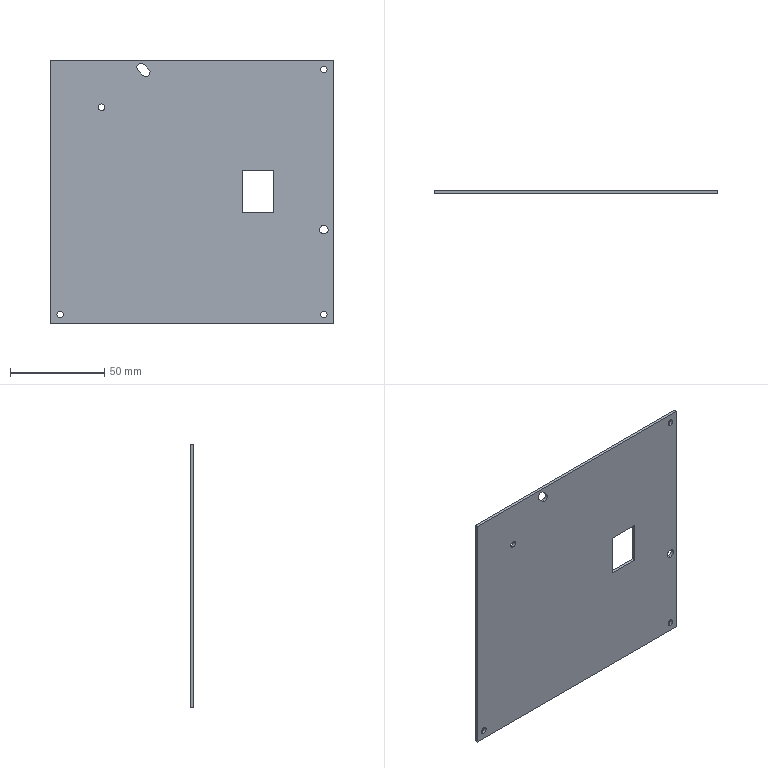Part | SolidWorks | features BaseBody 1 | 1 solid | 25 faces | box 150 x 1.6 x 140 mm | volume 32858 mm3 | cylinder 13 | plane 12 | commonest cylinder face diameters 3.5 x8 4.5 x5
STEP:
#1=CARTESIAN_POINT('',(12.475,-33.01,70.275));
#2=VERTEX_POINT('',#1);
#3=CARTESIAN_POINT('',(14.066,-33.01,74.116));
#4=VERTEX_POINT('',#3);
#5=CARTESIAN_POINT('',(12.475,-33.01,72.525));
#6=DIRECTION('',(0.,-1.,0.));
#7=DIRECTION('',(0.,0.,-1.));
#8=AXIS2_PLACEMENT_3D('',#5,#6,#7);
#9=CIRCLE('',#8,2.25);
#10=EDGE_CURVE('',#2,#4,#9,.T.);
#11=ORIENTED_EDGE('',*,*,#10,.F.);
#12=CARTESIAN_POINT('',(12.475,-34.61,70.275));
#13=VERTEX_POINT('',#12);
#14=CARTESIAN_POINT('',(12.475,-34.61,70.275));
#15=DIRECTION('',(0.,-1.,0.));
#16=VECTOR('',#15,1000.);
#17=LINE('',#14,#16);
#18=EDGE_CURVE('',#2,#13,#17,.T.);
#19=ORIENTED_EDGE('',*,*,#18,.T.);
#20=CARTESIAN_POINT('',(14.066,-34.61,74.116));
#21=VERTEX_POINT('',#20);
#22=CARTESIAN_POINT('',(12.475,-34.61,72.525));
#23=DIRECTION('',(0.,1.,0.));
#24=DIRECTION('',(0.,0.,-1.));
#25=AXIS2_PLACEMENT_3D('',#22,#23,#24);
#26=CIRCLE('',#25,2.25);
#27=EDGE_CURVE('',#21,#13,#26,.T.);
#28=ORIENTED_EDGE('',*,*,#27,.F.);
#29=CARTESIAN_POINT('',(14.066,-34.61,74.116));
#30=DIRECTION('',(0.,1.,0.));
#31=VECTOR('',#30,1000.);
#32=LINE('',#29,#31);
#33=EDGE_CURVE('',#21,#4,#32,.T.);
#34=ORIENTED_EDGE('',*,*,#33,.T.);
#35=EDGE_LOOP('',(#11,#19,#28,#34));
#36=FACE_OUTER_BOUND('',#35,.T.);
#37=CARTESIAN_POINT('',(12.475,-34.61,72.525));
#38=DIRECTION('',(0.,-1.,0.));
#39=DIRECTION('',(0.,0.,-1.));
#40=AXIS2_PLACEMENT_3D('',#37,#38,#39);
#41=CYLINDRICAL_SURFACE('',#40,2.25);
#42=ADVANCED_FACE('',(#36),#41,.F.);
#43=CARTESIAN_POINT('',(107.,-33.01,-8.75));
#44=VERTEX_POINT('',#43);
#45=CARTESIAN_POINT('',(107.,-33.01,-13.25));
#46=VERTEX_POINT('',#45);
#47=CARTESIAN_POINT('',(107.,-33.01,-11.));
#48=DIRECTION('',(0.,-1.,0.));
#49=DIRECTION('',(0.,0.,-1.));
#50=AXIS2_PLACEMENT_3D('',#47,#48,#49);
#51=CIRCLE('',#50,2.25);
#52=EDGE_CURVE('',#44,#46,#51,.T.);
#53=ORIENTED_EDGE('',*,*,#52,.F.);
#54=CARTESIAN_POINT('',(107.,-34.61,-8.75));
#55=VERTEX_POINT('',#54);
#56=CARTESIAN_POINT('',(107.,-34.61,-8.75));
#57=DIRECTION('',(0.,-1.,0.));
#58=VECTOR('',#57,1000.);
#59=LINE('',#56,#58);
#60=EDGE_CURVE('',#44,#55,#59,.T.);
#61=ORIENTED_EDGE('',*,*,#60,.T.);
#62=CARTESIAN_POINT('',(107.,-34.61,-13.25));
#63=VERTEX_POINT('',#62);
#64=CARTESIAN_POINT('',(107.,-34.61,-11.));
#65=DIRECTION('',(0.,1.,0.));
#66=DIRECTION('',(0.,0.,-1.));
#67=AXIS2_PLACEMENT_3D('',#64,#65,#66);
#68=CIRCLE('',#67,2.25);
#69=EDGE_CURVE('',#63,#55,#68,.T.);
#70=ORIENTED_EDGE('',*,*,#69,.F.);
#71=CARTESIAN_POINT('',(107.,-34.61,-13.25));
#72=DIRECTION('',(0.,-1.,0.));
#73=VECTOR('',#72,1000.);
#74=LINE('',#71,#73);
#75=EDGE_CURVE('',#46,#63,#74,.T.);
#76=ORIENTED_EDGE('',*,*,#75,.F.);
#77=EDGE_LOOP('',(#53,#61,#70,#76));
#78=FACE_OUTER_BOUND('',#77,.T.);
#79=CARTESIAN_POINT('',(107.,-34.61,-11.));
#80=DIRECTION('',(0.,-1.,0.));
#81=DIRECTION('',(0.,0.,-1.));
#82=AXIS2_PLACEMENT_3D('',#79,#80,#81);
#83=CYLINDRICAL_SURFACE('',#82,2.25);
#84=ADVANCED_FACE('',(#78),#83,.F.);
#85=CARTESIAN_POINT('',(107.,-33.01,75.75));
#86=VERTEX_POINT('',#85);
#87=CARTESIAN_POINT('',(107.,-33.01,72.25));
#88=VERTEX_POINT('',#87);
#89=CARTESIAN_POINT('',(107.,-33.01,74.));
#90=DIRECTION('',(0.,-1.,0.));
#91=DIRECTION('',(0.,0.,-1.));
#92=AXIS2_PLACEMENT_3D('',#89,#90,#91);
#93=CIRCLE('',#92,1.75);
#94=EDGE_CURVE('',#86,#88,#93,.T.);
#95=ORIENTED_EDGE('',*,*,#94,.F.);
#96=CARTESIAN_POINT('',(107.,-34.61,75.75));
#97=VERTEX_POINT('',#96);
#98=CARTESIAN_POINT('',(107.,-34.61,75.75));
#99=DIRECTION('',(0.,-1.,0.));
#100=VECTOR('',#99,1000.);
#101=LINE('',#98,#100);
#102=EDGE_CURVE('',#86,#97,#101,.T.);
#103=ORIENTED_EDGE('',*,*,#102,.T.);
#104=CARTESIAN_POINT('',(107.,-34.61,72.25));
#105=VERTEX_POINT('',#104);
#106=CARTESIAN_POINT('',(107.,-34.61,74.));
#107=DIRECTION('',(0.,1.,0.));
#108=DIRECTION('',(0.,0.,-1.));
#109=AXIS2_PLACEMENT_3D('',#106,#107,#108);
#110=CIRCLE('',#109,1.75);
#111=EDGE_CURVE('',#105,#97,#110,.T.);
#112=ORIENTED_EDGE('',*,*,#111,.F.);
#113=CARTESIAN_POINT('',(107.,-34.61,72.25));
#114=DIRECTION('',(0.,-1.,0.));
#115=VECTOR('',#114,1000.);
#116=LINE('',#113,#115);
#117=EDGE_CURVE('',#88,#105,#116,.T.);
#118=ORIENTED_EDGE('',*,*,#117,.F.);
#119=EDGE_LOOP('',(#95,#103,#112,#118));
#120=FACE_OUTER_BOUND('',#119,.T.);
#121=CARTESIAN_POINT('',(107.,-34.61,74.));
#122=DIRECTION('',(0.,-1.,0.));
#123=DIRECTION('',(0.,0.,-1.));
#124=AXIS2_PLACEMENT_3D('',#121,#122,#123);
#125=CYLINDRICAL_SURFACE('',#124,1.75);
#126=ADVANCED_FACE('',(#120),#125,.F.);
#127=CARTESIAN_POINT('',(-11.,-33.01,55.75));
#128=VERTEX_POINT('',#127);
#129=CARTESIAN_POINT('',(-11.,-33.01,52.25));
#130=VERTEX_POINT('',#129);
#131=CARTESIAN_POINT('',(-11.,-33.01,54.));
#132=DIRECTION('',(0.,-1.,0.));
#133=DIRECTION('',(0.,0.,-1.));
#134=AXIS2_PLACEMENT_3D('',#131,#132,#133);
#135=CIRCLE('',#134,1.75);
#136=EDGE_CURVE('',#128,#130,#135,.T.);
#137=ORIENTED_EDGE('',*,*,#136,.F.);
#138=CARTESIAN_POINT('',(-11.,-34.61,55.75));
#139=VERTEX_POINT('',#138);
#140=CARTESIAN_POINT('',(-11.,-34.61,55.75));
#141=DIRECTION('',(0.,-1.,0.));
#142=VECTOR('',#141,1000.);
#143=LINE('',#140,#142);
#144=EDGE_CURVE('',#128,#139,#143,.T.);
#145=ORIENTED_EDGE('',*,*,#144,.T.);
#146=CARTESIAN_POINT('',(-11.,-34.61,52.25));
#147=VERTEX_POINT('',#146);
#148=CARTESIAN_POINT('',(-11.,-34.61,54.));
#149=DIRECTION('',(0.,1.,0.));
#150=DIRECTION('',(0.,0.,-1.));
#151=AXIS2_PLACEMENT_3D('',#148,#149,#150);
#152=CIRCLE('',#151,1.75);
#153=EDGE_CURVE('',#147,#139,#152,.T.);
#154=ORIENTED_EDGE('',*,*,#153,.F.);
#155=CARTESIAN_POINT('',(-11.,-34.61,52.25));
#156=DIRECTION('',(0.,-1.,0.));
#157=VECTOR('',#156,1000.);
#158=LINE('',#155,#157);
#159=EDGE_CURVE('',#130,#147,#158,.T.);
#160=ORIENTED_EDGE('',*,*,#159,.F.);
#161=EDGE_LOOP('',(#137,#145,#154,#160));
#162=FACE_OUTER_BOUND('',#161,.T.);
#163=CARTESIAN_POINT('',(-11.,-34.61,54.));
#164=DIRECTION('',(0.,-1.,0.));
#165=DIRECTION('',(0.,0.,-1.));
#166=AXIS2_PLACEMENT_3D('',#163,#164,#165);
#167=CYLINDRICAL_SURFACE('',#166,1.75);
#168=ADVANCED_FACE('',(#162),#167,.F.);
#169=CARTESIAN_POINT('',(107.,-33.01,-54.25));
#170=VERTEX_POINT('',#169);
#171=CARTESIAN_POINT('',(107.,-33.01,-57.75));
#172=VERTEX_POINT('',#171);
#173=CARTESIAN_POINT('',(107.,-33.01,-56.));
#174=DIRECTION('',(0.,-1.,0.));
#175=DIRECTION('',(0.,0.,-1.));
#176=AXIS2_PLACEMENT_3D('',#173,#174,#175);
#177=CIRCLE('',#176,1.75);
#178=EDGE_CURVE('',#170,#172,#177,.T.);
#179=ORIENTED_EDGE('',*,*,#178,.F.);
#180=CARTESIAN_POINT('',(107.,-34.61,-54.25));
#181=VERTEX_POINT('',#180);
#182=CARTESIAN_POINT('',(107.,-34.61,-54.25));
#183=DIRECTION('',(0.,-1.,0.));
#184=VECTOR('',#183,1000.);
#185=LINE('',#182,#184);
#186=EDGE_CURVE('',#170,#181,#185,.T.);
#187=ORIENTED_EDGE('',*,*,#186,.T.);
#188=CARTESIAN_POINT('',(107.,-34.61,-57.75));
#189=VERTEX_POINT('',#188);
#190=CARTESIAN_POINT('',(107.,-34.61,-56.));
#191=DIRECTION('',(0.,1.,0.));
#192=DIRECTION('',(0.,0.,-1.));
#193=AXIS2_PLACEMENT_3D('',#190,#191,#192);
#194=CIRCLE('',#193,1.75);
#195=EDGE_CURVE('',#189,#181,#194,.T.);
#196=ORIENTED_EDGE('',*,*,#195,.F.);
#197=CARTESIAN_POINT('',(107.,-34.61,-57.75));
#198=DIRECTION('',(0.,-1.,0.));
#199=VECTOR('',#198,1000.);
#200=LINE('',#197,#199);
#201=EDGE_CURVE('',#172,#189,#200,.T.);
#202=ORIENTED_EDGE('',*,*,#201,.F.);
#203=EDGE_LOOP('',(#179,#187,#196,#202));
#204=FACE_OUTER_BOUND('',#203,.T.);
#205=CARTESIAN_POINT('',(107.,-34.61,-56.));
#206=DIRECTION('',(0.,-1.,0.));
#207=DIRECTION('',(0.,0.,-1.));
#208=AXIS2_PLACEMENT_3D('',#205,#206,#207);
#209=CYLINDRICAL_SURFACE('',#208,1.75);
#210=ADVANCED_FACE('',(#204),#209,.F.);
#211=CARTESIAN_POINT('',(-33.,-33.01,-54.25));
#212=VERTEX_POINT('',#211);
#213=CARTESIAN_POINT('',(-33.,-33.01,-57.75));
#214=VERTEX_POINT('',#213);
#215=CARTESIAN_POINT('',(-33.,-33.01,-56.));
#216=DIRECTION('',(0.,-1.,0.));
#217=DIRECTION('',(0.,0.,-1.));
#218=AXIS2_PLACEMENT_3D('',#215,#216,#217);
#219=CIRCLE('',#218,1.75);
#220=EDGE_CURVE('',#212,#214,#219,.T.);
#221=ORIENTED_EDGE('',*,*,#220,.F.);
#222=CARTESIAN_POINT('',(-33.,-34.61,-54.25));
#223=VERTEX_POINT('',#222);
#224=CARTESIAN_POINT('',(-33.,-34.61,-54.25));
#225=DIRECTION('',(0.,-1.,0.));
#226=VECTOR('',#225,1000.);
#227=LINE('',#224,#226);
#228=EDGE_CURVE('',#212,#223,#227,.T.);
#229=ORIENTED_EDGE('',*,*,#228,.T.);
#230=CARTESIAN_POINT('',(-33.,-34.61,-57.75));
#231=VERTEX_POINT('',#230);
#232=CARTESIAN_POINT('',(-33.,-34.61,-56.));
#233=DIRECTION('',(0.,1.,0.));
#234=DIRECTION('',(0.,0.,-1.));
#235=AXIS2_PLACEMENT_3D('',#232,#233,#234);
#236=CIRCLE('',#235,1.75);
#237=EDGE_CURVE('',#231,#223,#236,.T.);
#238=ORIENTED_EDGE('',*,*,#237,.F.);
#239=CARTESIAN_POINT('',(-33.,-34.61,-57.75));
#240=DIRECTION('',(0.,-1.,0.));
#241=VECTOR('',#240,1000.);
#242=LINE('',#239,#241);
#243=EDGE_CURVE('',#214,#231,#242,.T.);
#244=ORIENTED_EDGE('',*,*,#243,.F.);
#245=EDGE_LOOP('',(#221,#229,#238,#244));
#246=FACE_OUTER_BOUND('',#245,.T.);
#247=CARTESIAN_POINT('',(-33.,-34.61,-56.));
#248=DIRECTION('',(0.,-1.,0.));
#249=DIRECTION('',(0.,0.,-1.));
#250=AXIS2_PLACEMENT_3D('',#247,#248,#249);
#251=CYLINDRICAL_SURFACE('',#250,1.75);
#252=ADVANCED_FACE('',(#246),#251,.F.);
#253=CARTESIAN_POINT('',(80.34,-33.01,20.668));
#254=VERTEX_POINT('',#253);
#255=CARTESIAN_POINT('',(63.64,-33.01,20.668));
#256=VERTEX_POINT('',#255);
#257=CARTESIAN_POINT('',(18.5,-33.01,20.668));
#258=DIRECTION('',(-1.,0.,0.));
#259=VECTOR('',#258,1000.);
#260=LINE('',#257,#259);
#261=EDGE_CURVE('',#254,#256,#260,.T.);
#262=ORIENTED_EDGE('',*,*,#261,.T.);
#263=CARTESIAN_POINT('',(63.64,-33.01,-1.932));
#264=VERTEX_POINT('',#263);
#265=CARTESIAN_POINT('',(63.64,-33.01,24.));
#266=DIRECTION('',(0.,0.,-1.));
#267=VECTOR('',#266,1000.);
#268=LINE('',#265,#267);
#269=EDGE_CURVE('',#256,#264,#268,.T.);
#270=ORIENTED_EDGE('',*,*,#269,.T.);
#271=CARTESIAN_POINT('',(80.34,-33.01,-1.932));
#272=VERTEX_POINT('',#271);
#273=CARTESIAN_POINT('',(18.5,-33.01,-1.932));
#274=DIRECTION('',(1.,0.,0.));
#275=VECTOR('',#274,1000.);
#276=LINE('',#273,#275);
#277=EDGE_CURVE('',#264,#272,#276,.T.);
#278=ORIENTED_EDGE('',*,*,#277,.T.);
#279=CARTESIAN_POINT('',(80.34,-33.01,24.));
#280=DIRECTION('',(0.,0.,1.));
#281=VECTOR('',#280,1000.);
#282=LINE('',#279,#281);
#283=EDGE_CURVE('',#272,#254,#282,.T.);
#284=ORIENTED_EDGE('',*,*,#283,.T.);
#285=EDGE_LOOP('',(#262,#270,#278,#284));
#286=FACE_BOUND('',#285,.T.);
#287=CARTESIAN_POINT('',(11.591,-33.01,76.591));
#288=VERTEX_POINT('',#287);
#289=CARTESIAN_POINT('',(14.066,-33.01,74.116));
#290=DIRECTION('',(-0.7071,0.,0.7071));
#291=VECTOR('',#290,1000.);
#292=LINE('',#289,#291);
#293=EDGE_CURVE('',#4,#288,#292,.T.);
#294=ORIENTED_EDGE('',*,*,#293,.T.);
#295=CARTESIAN_POINT('',(8.409,-33.01,73.409));
#296=VERTEX_POINT('',#295);
#297=CARTESIAN_POINT('',(10.,-33.01,75.));
#298=DIRECTION('',(0.,-1.,0.));
#299=DIRECTION('',(0.,0.,-1.));
#300=AXIS2_PLACEMENT_3D('',#297,#298,#299);
#301=CIRCLE('',#300,2.25);
#302=EDGE_CURVE('',#288,#296,#301,.T.);
#303=ORIENTED_EDGE('',*,*,#302,.T.);
#304=CARTESIAN_POINT('',(10.884,-33.01,70.934));
#305=VERTEX_POINT('',#304);
#306=CARTESIAN_POINT('',(8.409,-33.01,73.409));
#307=DIRECTION('',(0.7071,0.,-0.7071));
#308=VECTOR('',#307,1000.);
#309=LINE('',#306,#308);
#310=EDGE_CURVE('',#296,#305,#309,.T.);
#311=ORIENTED_EDGE('',*,*,#310,.T.);
#312=CARTESIAN_POINT('',(12.475,-33.01,72.525));
#313=DIRECTION('',(0.,-1.,0.));
#314=DIRECTION('',(0.,0.,-1.));
#315=AXIS2_PLACEMENT_3D('',#312,#313,#314);
#316=CIRCLE('',#315,2.25);
#317=EDGE_CURVE('',#305,#2,#316,.T.);
#318=ORIENTED_EDGE('',*,*,#317,.T.);
#319=ORIENTED_EDGE('',*,*,#10,.T.);
#320=EDGE_LOOP('',(#294,#303,#311,#318,#319));
#321=FACE_BOUND('',#320,.T.);
#322=CARTESIAN_POINT('',(107.,-33.01,-11.));
#323=DIRECTION('',(0.,-1.,0.));
#324=DIRECTION('',(0.,0.,-1.));
#325=AXIS2_PLACEMENT_3D('',#322,#323,#324);
#326=CIRCLE('',#325,2.25);
#327=EDGE_CURVE('',#46,#44,#326,.T.);
#328=ORIENTED_EDGE('',*,*,#327,.T.);
#329=ORIENTED_EDGE('',*,*,#52,.T.);
#330=EDGE_LOOP('',(#328,#329));
#331=FACE_BOUND('',#330,.T.);
#332=CARTESIAN_POINT('',(107.,-33.01,74.));
#333=DIRECTION('',(0.,-1.,0.));
#334=DIRECTION('',(0.,0.,-1.));
#335=AXIS2_PLACEMENT_3D('',#332,#333,#334);
#336=CIRCLE('',#335,1.75);
#337=EDGE_CURVE('',#88,#86,#336,.T.);
#338=ORIENTED_EDGE('',*,*,#337,.T.);
#339=ORIENTED_EDGE('',*,*,#94,.T.);
#340=EDGE_LOOP('',(#338,#339));
#341=FACE_BOUND('',#340,.T.);
#342=CARTESIAN_POINT('',(-11.,-33.01,54.));
#343=DIRECTION('',(0.,-1.,0.));
#344=DIRECTION('',(0.,0.,-1.));
#345=AXIS2_PLACEMENT_3D('',#342,#343,#344);
#346=CIRCLE('',#345,1.75);
#347=EDGE_CURVE('',#130,#128,#346,.T.);
#348=ORIENTED_EDGE('',*,*,#347,.T.);
#349=ORIENTED_EDGE('',*,*,#136,.T.);
#350=EDGE_LOOP('',(#348,#349));
#351=FACE_BOUND('',#350,.T.);
#352=CARTESIAN_POINT('',(107.,-33.01,-56.));
#353=DIRECTION('',(0.,-1.,0.));
#354=DIRECTION('',(0.,0.,-1.));
#355=AXIS2_PLACEMENT_3D('',#352,#353,#354);
#356=CIRCLE('',#355,1.75);
#357=EDGE_CURVE('',#172,#170,#356,.T.);
#358=ORIENTED_EDGE('',*,*,#357,.T.);
#359=ORIENTED_EDGE('',*,*,#178,.T.);
#360=EDGE_LOOP('',(#358,#359));
#361=FACE_BOUND('',#360,.T.);
#362=CARTESIAN_POINT('',(-33.,-33.01,-56.));
#363=DIRECTION('',(0.,-1.,0.));
#364=DIRECTION('',(0.,0.,-1.));
#365=AXIS2_PLACEMENT_3D('',#362,#363,#364);
#366=CIRCLE('',#365,1.75);
#367=EDGE_CURVE('',#214,#212,#366,.T.);
#368=ORIENTED_EDGE('',*,*,#367,.T.);
#369=ORIENTED_EDGE('',*,*,#220,.T.);
#370=EDGE_LOOP('',(#368,#369));
#371=FACE_BOUND('',#370,.T.);
#372=CARTESIAN_POINT('',(112.,-33.01,-61.));
#373=VERTEX_POINT('',#372);
#374=CARTESIAN_POINT('',(-38.,-33.01,-61.));
#375=VERTEX_POINT('',#374);
#376=CARTESIAN_POINT('',(18.5,-33.01,-61.));
#377=DIRECTION('',(-1.,0.,0.));
#378=VECTOR('',#377,1000.);
#379=LINE('',#376,#378);
#380=EDGE_CURVE('',#373,#375,#379,.T.);
#381=ORIENTED_EDGE('',*,*,#380,.T.);
#382=CARTESIAN_POINT('',(-38.,-33.01,79.));
#383=VERTEX_POINT('',#382);
#384=CARTESIAN_POINT('',(-38.,-33.01,24.));
#385=DIRECTION('',(0.,0.,1.));
#386=VECTOR('',#385,1000.);
#387=LINE('',#384,#386);
#388=EDGE_CURVE('',#375,#383,#387,.T.);
#389=ORIENTED_EDGE('',*,*,#388,.T.);
#390=CARTESIAN_POINT('',(112.,-33.01,79.));
#391=VERTEX_POINT('',#390);
#392=CARTESIAN_POINT('',(18.5,-33.01,79.));
#393=DIRECTION('',(1.,0.,0.));
#394=VECTOR('',#393,1000.);
#395=LINE('',#392,#394);
#396=EDGE_CURVE('',#383,#391,#395,.T.);
#397=ORIENTED_EDGE('',*,*,#396,.T.);
#398=CARTESIAN_POINT('',(112.,-33.01,24.));
#399=DIRECTION('',(0.,0.,-1.));
#400=VECTOR('',#399,1000.);
#401=LINE('',#398,#400);
#402=EDGE_CURVE('',#391,#373,#401,.T.);
#403=ORIENTED_EDGE('',*,*,#402,.T.);
#404=EDGE_LOOP('',(#381,#389,#397,#403));
#405=FACE_OUTER_BOUND('',#404,.T.);
#406=CARTESIAN_POINT('',(18.5,-33.01,24.));
#407=DIRECTION('',(0.,1.,0.));
#408=DIRECTION('',(0.,0.,1.));
#409=AXIS2_PLACEMENT_3D('',#406,#407,#408);
#410=PLANE('',#409);
#411=ADVANCED_FACE('',(#286,#321,#331,#341,#351,#361,#371,#405),#410,.T.);
#412=CARTESIAN_POINT('',(63.64,-34.61,-1.932));
#413=VERTEX_POINT('',#412);
#414=CARTESIAN_POINT('',(63.64,-34.61,20.668));
#415=VERTEX_POINT('',#414);
#416=CARTESIAN_POINT('',(63.64,-34.61,20.668));
#417=DIRECTION('',(0.,0.,1.));
#418=VECTOR('',#417,1000.);
#419=LINE('',#416,#418);
#420=EDGE_CURVE('',#413,#415,#419,.T.);
#421=ORIENTED_EDGE('',*,*,#420,.F.);
#422=CARTESIAN_POINT('',(63.64,-34.61,-1.932));
#423=DIRECTION('',(0.,-1.,0.));
#424=VECTOR('',#423,1000.);
#425=LINE('',#422,#424);
#426=EDGE_CURVE('',#264,#413,#425,.T.);
#427=ORIENTED_EDGE('',*,*,#426,.F.);
#428=ORIENTED_EDGE('',*,*,#269,.F.);
#429=CARTESIAN_POINT('',(63.64,-34.61,20.668));
#430=DIRECTION('',(0.,1.,0.));
#431=VECTOR('',#430,1000.);
#432=LINE('',#429,#431);
#433=EDGE_CURVE('',#415,#256,#432,.T.);
#434=ORIENTED_EDGE('',*,*,#433,.F.);
#435=EDGE_LOOP('',(#421,#427,#428,#434));
#436=FACE_OUTER_BOUND('',#435,.T.);
#437=CARTESIAN_POINT('',(63.64,-34.61,20.668));
#438=DIRECTION('',(-1.,0.,0.));
#439=DIRECTION('',(0.,0.,1.));
#440=AXIS2_PLACEMENT_3D('',#437,#438,#439);
#441=PLANE('',#440);
#442=ADVANCED_FACE('',(#436),#441,.F.);
#443=CARTESIAN_POINT('',(80.34,-34.61,20.668));
#444=VERTEX_POINT('',#443);
#445=CARTESIAN_POINT('',(80.34,-34.61,20.668));
#446=DIRECTION('',(1.,0.,0.));
#447=VECTOR('',#446,1000.);
#448=LINE('',#445,#447);
#449=EDGE_CURVE('',#415,#444,#448,.T.);
#450=ORIENTED_EDGE('',*,*,#449,.F.);
#451=ORIENTED_EDGE('',*,*,#433,.T.);
#452=ORIENTED_EDGE('',*,*,#261,.F.);
#453=CARTESIAN_POINT('',(80.34,-34.61,20.668));
#454=DIRECTION('',(0.,1.,0.));
#455=VECTOR('',#454,1000.);
#456=LINE('',#453,#455);
#457=EDGE_CURVE('',#444,#254,#456,.T.);
#458=ORIENTED_EDGE('',*,*,#457,.F.);
#459=EDGE_LOOP('',(#450,#451,#452,#458));
#460=FACE_OUTER_BOUND('',#459,.T.);
#461=CARTESIAN_POINT('',(80.34,-34.61,20.668));
#462=DIRECTION('',(0.,0.,1.));
#463=DIRECTION('',(1.,0.,0.));
#464=AXIS2_PLACEMENT_3D('',#461,#462,#463);
#465=PLANE('',#464);
#466=ADVANCED_FACE('',(#460),#465,.F.);
#467=CARTESIAN_POINT('',(80.34,-34.61,-1.932));
#468=VERTEX_POINT('',#467);
#469=CARTESIAN_POINT('',(80.34,-34.61,-1.932));
#470=DIRECTION('',(0.,0.,-1.));
#471=VECTOR('',#470,1000.);
#472=LINE('',#469,#471);
#473=EDGE_CURVE('',#444,#468,#472,.T.);
#474=ORIENTED_EDGE('',*,*,#473,.F.);
#475=ORIENTED_EDGE('',*,*,#457,.T.);
#476=ORIENTED_EDGE('',*,*,#283,.F.);
#477=CARTESIAN_POINT('',(80.34,-34.61,-1.932));
#478=DIRECTION('',(0.,1.,0.));
#479=VECTOR('',#478,1000.);
#480=LINE('',#477,#479);
#481=EDGE_CURVE('',#468,#272,#480,.T.);
#482=ORIENTED_EDGE('',*,*,#481,.F.);
#483=EDGE_LOOP('',(#474,#475,#476,#482));
#484=FACE_OUTER_BOUND('',#483,.T.);
#485=CARTESIAN_POINT('',(80.34,-34.61,-1.932));
#486=DIRECTION('',(1.,0.,0.));
#487=DIRECTION('',(0.,0.,-1.));
#488=AXIS2_PLACEMENT_3D('',#485,#486,#487);
#489=PLANE('',#488);
#490=ADVANCED_FACE('',(#484),#489,.F.);
#491=CARTESIAN_POINT('',(63.64,-34.61,-1.932));
#492=DIRECTION('',(-1.,0.,0.));
#493=VECTOR('',#492,1000.);
#494=LINE('',#491,#493);
#495=EDGE_CURVE('',#468,#413,#494,.T.);
#496=ORIENTED_EDGE('',*,*,#495,.F.);
#497=ORIENTED_EDGE('',*,*,#481,.T.);
#498=ORIENTED_EDGE('',*,*,#277,.F.);
#499=ORIENTED_EDGE('',*,*,#426,.T.);
#500=EDGE_LOOP('',(#496,#497,#498,#499));
#501=FACE_OUTER_BOUND('',#500,.T.);
#502=CARTESIAN_POINT('',(63.64,-34.61,-1.932));
#503=DIRECTION('',(0.,0.,-1.));
#504=DIRECTION('',(-1.,0.,0.));
#505=AXIS2_PLACEMENT_3D('',#502,#503,#504);
#506=PLANE('',#505);
#507=ADVANCED_FACE('',(#501),#506,.F.);
#508=CARTESIAN_POINT('',(8.409,-34.61,73.409));
#509=VERTEX_POINT('',#508);
#510=CARTESIAN_POINT('',(11.591,-34.61,76.591));
#511=VERTEX_POINT('',#510);
#512=CARTESIAN_POINT('',(10.,-34.61,75.));
#513=DIRECTION('',(0.,1.,0.));
#514=DIRECTION('',(0.,0.,-1.));
#515=AXIS2_PLACEMENT_3D('',#512,#513,#514);
#516=CIRCLE('',#515,2.25);
#517=EDGE_CURVE('',#509,#511,#516,.T.);
#518=ORIENTED_EDGE('',*,*,#517,.F.);
#519=CARTESIAN_POINT('',(8.409,-34.61,73.409));
#520=DIRECTION('',(0.,-1.,0.));
#521=VECTOR('',#520,1000.);
#522=LINE('',#519,#521);
#523=EDGE_CURVE('',#296,#509,#522,.T.);
#524=ORIENTED_EDGE('',*,*,#523,.F.);
#525=ORIENTED_EDGE('',*,*,#302,.F.);
#526=CARTESIAN_POINT('',(11.591,-34.61,76.591));
#527=DIRECTION('',(0.,1.,0.));
#528=VECTOR('',#527,1000.);
#529=LINE('',#526,#528);
#530=EDGE_CURVE('',#511,#288,#529,.T.);
#531=ORIENTED_EDGE('',*,*,#530,.F.);
#532=EDGE_LOOP('',(#518,#524,#525,#531));
#533=FACE_OUTER_BOUND('',#532,.T.);
#534=CARTESIAN_POINT('',(10.,-34.61,75.));
#535=DIRECTION('',(0.,-1.,0.));
#536=DIRECTION('',(0.,0.,-1.));
#537=AXIS2_PLACEMENT_3D('',#534,#535,#536);
#538=CYLINDRICAL_SURFACE('',#537,2.25);
#539=ADVANCED_FACE('',(#533),#538,.F.);
#540=CARTESIAN_POINT('',(14.066,-34.61,74.116));
#541=DIRECTION('',(0.7071,0.,-0.7071));
#542=VECTOR('',#541,1000.);
#543=LINE('',#540,#542);
#544=EDGE_CURVE('',#511,#21,#543,.T.);
#545=ORIENTED_EDGE('',*,*,#544,.F.);
#546=ORIENTED_EDGE('',*,*,#530,.T.);
#547=ORIENTED_EDGE('',*,*,#293,.F.);
#548=ORIENTED_EDGE('',*,*,#33,.F.);
#549=EDGE_LOOP('',(#545,#546,#547,#548));
#550=FACE_OUTER_BOUND('',#549,.T.);
#551=CARTESIAN_POINT('',(14.066,-34.61,74.116));
#552=DIRECTION('',(0.7071,0.,0.7071));
#553=DIRECTION('',(0.7071,0.,-0.7071));
#554=AXIS2_PLACEMENT_3D('',#551,#552,#553);
#555=PLANE('',#554);
#556=ADVANCED_FACE('',(#550),#555,.F.);
#557=ORIENTED_EDGE('',*,*,#18,.F.);
#558=ORIENTED_EDGE('',*,*,#317,.F.);
#559=CARTESIAN_POINT('',(10.884,-34.61,70.934));
#560=VERTEX_POINT('',#559);
#561=CARTESIAN_POINT('',(10.884,-34.61,70.934));
#562=DIRECTION('',(0.,1.,0.));
#563=VECTOR('',#562,1000.);
#564=LINE('',#561,#563);
#565=EDGE_CURVE('',#560,#305,#564,.T.);
#566=ORIENTED_EDGE('',*,*,#565,.F.);
#567=CARTESIAN_POINT('',(12.475,-34.61,72.525));
#568=DIRECTION('',(0.,1.,0.));
#569=DIRECTION('',(0.,0.,-1.));
#570=AXIS2_PLACEMENT_3D('',#567,#568,#569);
#571=CIRCLE('',#570,2.25);
#572=EDGE_CURVE('',#13,#560,#571,.T.);
#573=ORIENTED_EDGE('',*,*,#572,.F.);
#574=EDGE_LOOP('',(#557,#558,#566,#573));
#575=FACE_OUTER_BOUND('',#574,.T.);
#576=CARTESIAN_POINT('',(12.475,-34.61,72.525));
#577=DIRECTION('',(0.,-1.,0.));
#578=DIRECTION('',(0.,0.,-1.));
#579=AXIS2_PLACEMENT_3D('',#576,#577,#578);
#580=CYLINDRICAL_SURFACE('',#579,2.25);
#581=ADVANCED_FACE('',(#575),#580,.F.);
#582=CARTESIAN_POINT('',(8.409,-34.61,73.409));
#583=DIRECTION('',(-0.7071,0.,0.7071));
#584=VECTOR('',#583,1000.);
#585=LINE('',#582,#584);
#586=EDGE_CURVE('',#560,#509,#585,.T.);
#587=ORIENTED_EDGE('',*,*,#586,.F.);
#588=ORIENTED_EDGE('',*,*,#565,.T.);
#589=ORIENTED_EDGE('',*,*,#310,.F.);
#590=ORIENTED_EDGE('',*,*,#523,.T.);
#591=EDGE_LOOP('',(#587,#588,#589,#590));
#592=FACE_OUTER_BOUND('',#591,.T.);
#593=CARTESIAN_POINT('',(8.409,-34.61,73.409));
#594=DIRECTION('',(-0.7071,0.,-0.7071));
#595=DIRECTION('',(-0.7071,0.,0.7071));
#596=AXIS2_PLACEMENT_3D('',#593,#594,#595);
#597=PLANE('',#596);
#598=ADVANCED_FACE('',(#592),#597,.F.);
#599=ORIENTED_EDGE('',*,*,#60,.F.);
#600=ORIENTED_EDGE('',*,*,#327,.F.);
#601=ORIENTED_EDGE('',*,*,#75,.T.);
#602=CARTESIAN_POINT('',(107.,-34.61,-11.));
#603=DIRECTION('',(0.,1.,0.));
#604=DIRECTION('',(0.,0.,-1.));
#605=AXIS2_PLACEMENT_3D('',#602,#603,#604);
#606=CIRCLE('',#605,2.25);
#607=EDGE_CURVE('',#55,#63,#606,.T.);
#608=ORIENTED_EDGE('',*,*,#607,.F.);
#609=EDGE_LOOP('',(#599,#600,#601,#608));
#610=FACE_OUTER_BOUND('',#609,.T.);
#611=CARTESIAN_POINT('',(107.,-34.61,-11.));
#612=DIRECTION('',(0.,-1.,0.));
#613=DIRECTION('',(0.,0.,-1.));
#614=AXIS2_PLACEMENT_3D('',#611,#612,#613);
#615=CYLINDRICAL_SURFACE('',#614,2.25);
#616=ADVANCED_FACE('',(#610),#615,.F.);
#617=ORIENTED_EDGE('',*,*,#102,.F.);
#618=ORIENTED_EDGE('',*,*,#337,.F.);
#619=ORIENTED_EDGE('',*,*,#117,.T.);
#620=CARTESIAN_POINT('',(107.,-34.61,74.));
#621=DIRECTION('',(0.,1.,0.));
#622=DIRECTION('',(0.,0.,-1.));
#623=AXIS2_PLACEMENT_3D('',#620,#621,#622);
#624=CIRCLE('',#623,1.75);
#625=EDGE_CURVE('',#97,#105,#624,.T.);
#626=ORIENTED_EDGE('',*,*,#625,.F.);
#627=EDGE_LOOP('',(#617,#618,#619,#626));
#628=FACE_OUTER_BOUND('',#627,.T.);
#629=CARTESIAN_POINT('',(107.,-34.61,74.));
#630=DIRECTION('',(0.,-1.,0.));
#631=DIRECTION('',(0.,0.,-1.));
#632=AXIS2_PLACEMENT_3D('',#629,#630,#631);
#633=CYLINDRICAL_SURFACE('',#632,1.75);
#634=ADVANCED_FACE('',(#628),#633,.F.);
#635=ORIENTED_EDGE('',*,*,#144,.F.);
#636=ORIENTED_EDGE('',*,*,#347,.F.);
#637=ORIENTED_EDGE('',*,*,#159,.T.);
#638=CARTESIAN_POINT('',(-11.,-34.61,54.));
#639=DIRECTION('',(0.,1.,0.));
#640=DIRECTION('',(0.,0.,-1.));
#641=AXIS2_PLACEMENT_3D('',#638,#639,#640);
#642=CIRCLE('',#641,1.75);
#643=EDGE_CURVE('',#139,#147,#642,.T.);
#644=ORIENTED_EDGE('',*,*,#643,.F.);
#645=EDGE_LOOP('',(#635,#636,#637,#644));
#646=FACE_OUTER_BOUND('',#645,.T.);
#647=CARTESIAN_POINT('',(-11.,-34.61,54.));
#648=DIRECTION('',(0.,-1.,0.));
#649=DIRECTION('',(0.,0.,-1.));
#650=AXIS2_PLACEMENT_3D('',#647,#648,#649);
#651=CYLINDRICAL_SURFACE('',#650,1.75);
#652=ADVANCED_FACE('',(#646),#651,.F.);
#653=ORIENTED_EDGE('',*,*,#186,.F.);
#654=ORIENTED_EDGE('',*,*,#357,.F.);
#655=ORIENTED_EDGE('',*,*,#201,.T.);
#656=CARTESIAN_POINT('',(107.,-34.61,-56.));
#657=DIRECTION('',(0.,1.,0.));
#658=DIRECTION('',(0.,0.,-1.));
#659=AXIS2_PLACEMENT_3D('',#656,#657,#658);
#660=CIRCLE('',#659,1.75);
#661=EDGE_CURVE('',#181,#189,#660,.T.);
#662=ORIENTED_EDGE('',*,*,#661,.F.);
#663=EDGE_LOOP('',(#653,#654,#655,#662));
#664=FACE_OUTER_BOUND('',#663,.T.);
#665=CARTESIAN_POINT('',(107.,-34.61,-56.));
#666=DIRECTION('',(0.,-1.,0.));
#667=DIRECTION('',(0.,0.,-1.));
#668=AXIS2_PLACEMENT_3D('',#665,#666,#667);
#669=CYLINDRICAL_SURFACE('',#668,1.75);
#670=ADVANCED_FACE('',(#664),#669,.F.);
#671=ORIENTED_EDGE('',*,*,#228,.F.);
#672=ORIENTED_EDGE('',*,*,#367,.F.);
#673=ORIENTED_EDGE('',*,*,#243,.T.);
#674=CARTESIAN_POINT('',(-33.,-34.61,-56.));
#675=DIRECTION('',(0.,1.,0.));
#676=DIRECTION('',(0.,0.,-1.));
#677=AXIS2_PLACEMENT_3D('',#674,#675,#676);
#678=CIRCLE('',#677,1.75);
#679=EDGE_CURVE('',#223,#231,#678,.T.);
#680=ORIENTED_EDGE('',*,*,#679,.F.);
#681=EDGE_LOOP('',(#671,#672,#673,#680));
#682=FACE_OUTER_BOUND('',#681,.T.);
#683=CARTESIAN_POINT('',(-33.,-34.61,-56.));
#684=DIRECTION('',(0.,-1.,0.));
#685=DIRECTION('',(0.,0.,-1.));
#686=AXIS2_PLACEMENT_3D('',#683,#684,#685);
#687=CYLINDRICAL_SURFACE('',#686,1.75);
#688=ADVANCED_FACE('',(#682),#687,.F.);
#689=ORIENTED_EDGE('',*,*,#388,.F.);
#690=CARTESIAN_POINT('',(-38.,-34.61,-61.));
#691=VERTEX_POINT('',#690);
#692=CARTESIAN_POINT('',(-38.,-34.61,-61.));
#693=DIRECTION('',(0.,1.,0.));
#694=VECTOR('',#693,1000.);
#695=LINE('',#692,#694);
#696=EDGE_CURVE('',#691,#375,#695,.T.);
#697=ORIENTED_EDGE('',*,*,#696,.F.);
#698=CARTESIAN_POINT('',(-38.,-34.61,79.));
#699=VERTEX_POINT('',#698);
#700=CARTESIAN_POINT('',(-38.,-34.61,-46.));
#701=DIRECTION('',(0.,0.,-1.));
#702=VECTOR('',#701,1000.);
#703=LINE('',#700,#702);
#704=EDGE_CURVE('',#699,#691,#703,.T.);
#705=ORIENTED_EDGE('',*,*,#704,.F.);
#706=CARTESIAN_POINT('',(-38.,-34.61,79.));
#707=DIRECTION('',(0.,-1.,0.));
#708=VECTOR('',#707,1000.);
#709=LINE('',#706,#708);
#710=EDGE_CURVE('',#383,#699,#709,.T.);
#711=ORIENTED_EDGE('',*,*,#710,.F.);
#712=EDGE_LOOP('',(#689,#697,#705,#711));
#713=FACE_OUTER_BOUND('',#712,.T.);
#714=CARTESIAN_POINT('',(-38.,-34.61,-46.));
#715=DIRECTION('',(1.,0.,0.));
#716=DIRECTION('',(0.,0.,-1.));
#717=AXIS2_PLACEMENT_3D('',#714,#715,#716);
#718=PLANE('',#717);
#719=ADVANCED_FACE('',(#713),#718,.F.);
#720=CARTESIAN_POINT('',(112.,-34.61,-61.));
#721=VERTEX_POINT('',#720);
#722=CARTESIAN_POINT('',(112.,-34.61,-61.));
#723=DIRECTION('',(0.,-1.,0.));
#724=VECTOR('',#723,1000.);
#725=LINE('',#722,#724);
#726=EDGE_CURVE('',#373,#721,#725,.T.);
#727=ORIENTED_EDGE('',*,*,#726,.T.);
#728=CARTESIAN_POINT('',(-38.,-34.61,-61.));
#729=DIRECTION('',(-1.,0.,0.));
#730=VECTOR('',#729,1000.);
#731=LINE('',#728,#730);
#732=EDGE_CURVE('',#721,#691,#731,.T.);
#733=ORIENTED_EDGE('',*,*,#732,.T.);
#734=ORIENTED_EDGE('',*,*,#696,.T.);
#735=ORIENTED_EDGE('',*,*,#380,.F.);
#736=EDGE_LOOP('',(#727,#733,#734,#735));
#737=FACE_OUTER_BOUND('',#736,.T.);
#738=CARTESIAN_POINT('',(-38.,-34.61,-61.));
#739=DIRECTION('',(0.,0.,-1.));
#740=DIRECTION('',(-1.,0.,0.));
#741=AXIS2_PLACEMENT_3D('',#738,#739,#740);
#742=PLANE('',#741);
#743=ADVANCED_FACE('',(#737),#742,.T.);
#744=ORIENTED_EDGE('',*,*,#726,.F.);
#745=ORIENTED_EDGE('',*,*,#402,.F.);
#746=CARTESIAN_POINT('',(112.,-34.61,79.));
#747=VERTEX_POINT('',#746);
#748=CARTESIAN_POINT('',(112.,-33.81,79.));
#749=DIRECTION('',(0.,-1.,0.));
#750=VECTOR('',#749,1000.);
#751=LINE('',#748,#750);
#752=EDGE_CURVE('',#391,#747,#751,.T.);
#753=ORIENTED_EDGE('',*,*,#752,.T.);
#754=CARTESIAN_POINT('',(112.,-34.61,21.5));
#755=DIRECTION('',(0.,0.,-1.));
#756=VECTOR('',#755,1000.);
#757=LINE('',#754,#756);
#758=EDGE_CURVE('',#747,#721,#757,.T.);
#759=ORIENTED_EDGE('',*,*,#758,.T.);
#760=EDGE_LOOP('',(#744,#745,#753,#759));
#761=FACE_OUTER_BOUND('',#760,.T.);
#762=CARTESIAN_POINT('',(112.,-33.81,21.5));
#763=DIRECTION('',(1.,0.,0.));
#764=DIRECTION('',(0.,0.,-1.));
#765=AXIS2_PLACEMENT_3D('',#762,#763,#764);
#766=PLANE('',#765);
#767=ADVANCED_FACE('',(#761),#766,.T.);
#768=ORIENTED_EDGE('',*,*,#396,.F.);
#769=ORIENTED_EDGE('',*,*,#710,.T.);
#770=CARTESIAN_POINT('',(-26.851,-34.61,79.));
#771=DIRECTION('',(1.,0.,0.));
#772=VECTOR('',#771,1000.);
#773=LINE('',#770,#772);
#774=EDGE_CURVE('',#699,#747,#773,.T.);
#775=ORIENTED_EDGE('',*,*,#774,.T.);
#776=ORIENTED_EDGE('',*,*,#752,.F.);
#777=EDGE_LOOP('',(#768,#769,#775,#776));
#778=FACE_OUTER_BOUND('',#777,.T.);
#779=CARTESIAN_POINT('',(-26.851,-33.81,79.));
#780=DIRECTION('',(0.,0.,1.));
#781=DIRECTION('',(1.,0.,0.));
#782=AXIS2_PLACEMENT_3D('',#779,#780,#781);
#783=PLANE('',#782);
#784=ADVANCED_FACE('',(#778),#783,.T.);
#785=ORIENTED_EDGE('',*,*,#473,.T.);
#786=ORIENTED_EDGE('',*,*,#495,.T.);
#787=ORIENTED_EDGE('',*,*,#420,.T.);
#788=ORIENTED_EDGE('',*,*,#449,.T.);
#789=EDGE_LOOP('',(#785,#786,#787,#788));
#790=FACE_BOUND('',#789,.T.);
#791=ORIENTED_EDGE('',*,*,#27,.T.);
#792=ORIENTED_EDGE('',*,*,#572,.T.);
#793=ORIENTED_EDGE('',*,*,#586,.T.);
#794=ORIENTED_EDGE('',*,*,#517,.T.);
#795=ORIENTED_EDGE('',*,*,#544,.T.);
#796=EDGE_LOOP('',(#791,#792,#793,#794,#795));
#797=FACE_BOUND('',#796,.T.);
#798=ORIENTED_EDGE('',*,*,#69,.T.);
#799=ORIENTED_EDGE('',*,*,#607,.T.);
#800=EDGE_LOOP('',(#798,#799));
#801=FACE_BOUND('',#800,.T.);
#802=ORIENTED_EDGE('',*,*,#111,.T.);
#803=ORIENTED_EDGE('',*,*,#625,.T.);
#804=EDGE_LOOP('',(#802,#803));
#805=FACE_BOUND('',#804,.T.);
#806=ORIENTED_EDGE('',*,*,#153,.T.);
#807=ORIENTED_EDGE('',*,*,#643,.T.);
#808=EDGE_LOOP('',(#806,#807));
#809=FACE_BOUND('',#808,.T.);
#810=ORIENTED_EDGE('',*,*,#195,.T.);
#811=ORIENTED_EDGE('',*,*,#661,.T.);
#812=EDGE_LOOP('',(#810,#811));
#813=FACE_BOUND('',#812,.T.);
#814=ORIENTED_EDGE('',*,*,#237,.T.);
#815=ORIENTED_EDGE('',*,*,#679,.T.);
#816=EDGE_LOOP('',(#814,#815));
#817=FACE_BOUND('',#816,.T.);
#818=ORIENTED_EDGE('',*,*,#704,.T.);
#819=ORIENTED_EDGE('',*,*,#732,.F.);
#820=ORIENTED_EDGE('',*,*,#758,.F.);
#821=ORIENTED_EDGE('',*,*,#774,.F.);
#822=EDGE_LOOP('',(#818,#819,#820,#821));
#823=FACE_OUTER_BOUND('',#822,.T.);
#824=CARTESIAN_POINT('',(18.5,-34.61,24.));
#825=DIRECTION('',(0.,1.,0.));
#826=DIRECTION('',(0.,0.,1.));
#827=AXIS2_PLACEMENT_3D('',#824,#825,#826);
#828=PLANE('',#827);
#829=ADVANCED_FACE('',(#790,#797,#801,#805,#809,#813,#817,#823),#828,.F.);
#830=CLOSED_SHELL('',(#42,#84,#126,#168,#210,#252,#411,#442,#466,#490,#507,#539,#556,#581,#598,#616,#634,#652,#670,#688,#719,#743,#767,#784,#829));
#831=MANIFOLD_SOLID_BREP('',#830);
#832=CARTESIAN_POINT('',(0.,0.,0.));
#833=DIRECTION('',(0.,0.,1.));
#834=DIRECTION('',(1.,0.,0.));
#835=AXIS2_PLACEMENT_3D('',#832,#833,#834);
#836=(LENGTH_UNIT()NAMED_UNIT(*)SI_UNIT(.MILLI.,.METRE.));
#837=UNCERTAINTY_MEASURE_WITH_UNIT(LENGTH_MEASURE(0.00001),#836,'','');
#838=(NAMED_UNIT(*)PLANE_ANGLE_UNIT()SI_UNIT($,.RADIAN.));
#839=(NAMED_UNIT(*)SI_UNIT($,.STERADIAN.)SOLID_ANGLE_UNIT());
#840=(GEOMETRIC_REPRESENTATION_CONTEXT(3)GLOBAL_UNCERTAINTY_ASSIGNED_CONTEXT((#837))GLOBAL_UNIT_ASSIGNED_CONTEXT((#836,#838,#839))REPRESENTATION_CONTEXT('',''));
#841=ADVANCED_BREP_SHAPE_REPRESENTATION('',(#831,#835),#840);